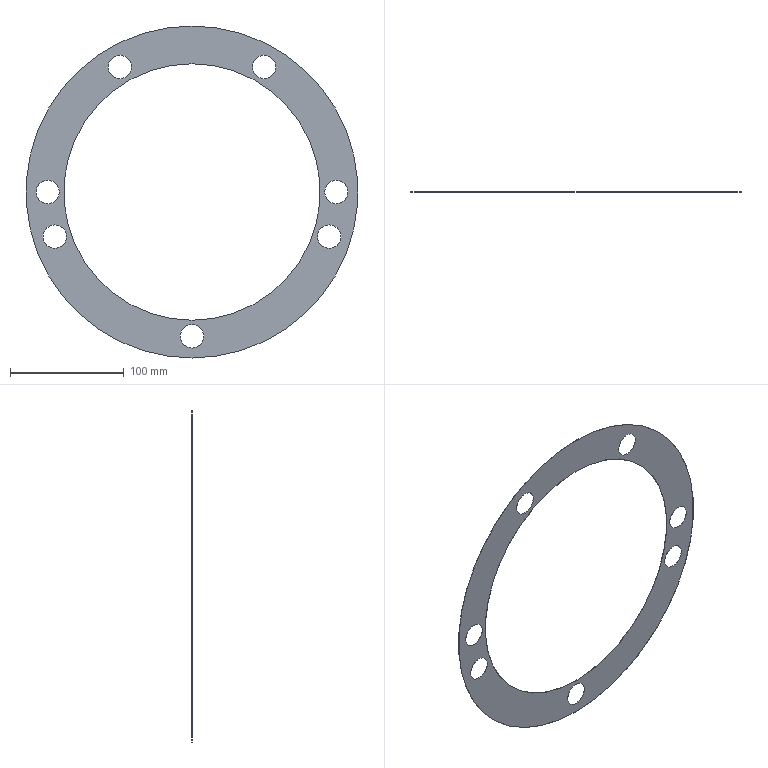Part | SolidWorks | features HoleWzd 2, Extrusion 1, MirrorPattern 1 | 1 solid | 20 faces | box 292.1 x 0.254 x 292.1 mm | volume 6277 mm3 | cylinder 18 | plane 2 | commonest cylinder face diameters 20.637 x14 225.552 x2 292.1 x2
STEP:
#1=CARTESIAN_POINT('',(-63.5,0.254,120.301));
#2=VERTEX_POINT('',#1);
#3=CARTESIAN_POINT('',(-63.5,0.254,99.663));
#4=VERTEX_POINT('',#3);
#5=CARTESIAN_POINT('',(-63.5,0.254,109.982));
#6=DIRECTION('',(0.,-1.,0.));
#7=DIRECTION('',(0.,0.,-1.));
#8=AXIS2_PLACEMENT_3D('',#5,#6,#7);
#9=CIRCLE('',#8,10.319);
#10=EDGE_CURVE('',#2,#4,#9,.T.);
#11=ORIENTED_EDGE('',*,*,#10,.F.);
#12=CARTESIAN_POINT('',(-63.5,0.,120.301));
#13=VERTEX_POINT('',#12);
#14=CARTESIAN_POINT('',(-63.5,0.,120.301));
#15=DIRECTION('',(0.,-1.,0.));
#16=VECTOR('',#15,1000.);
#17=LINE('',#14,#16);
#18=EDGE_CURVE('',#2,#13,#17,.T.);
#19=ORIENTED_EDGE('',*,*,#18,.T.);
#20=CARTESIAN_POINT('',(-63.5,0.,99.663));
#21=VERTEX_POINT('',#20);
#22=CARTESIAN_POINT('',(-63.5,0.,109.982));
#23=DIRECTION('',(0.,-1.,0.));
#24=DIRECTION('',(0.,0.,-1.));
#25=AXIS2_PLACEMENT_3D('',#22,#23,#24);
#26=CIRCLE('',#25,10.319);
#27=EDGE_CURVE('',#13,#21,#26,.T.);
#28=ORIENTED_EDGE('',*,*,#27,.T.);
#29=CARTESIAN_POINT('',(-63.5,0.,99.663));
#30=DIRECTION('',(0.,-1.,0.));
#31=VECTOR('',#30,1000.);
#32=LINE('',#29,#31);
#33=EDGE_CURVE('',#4,#21,#32,.T.);
#34=ORIENTED_EDGE('',*,*,#33,.F.);
#35=EDGE_LOOP('',(#11,#19,#28,#34));
#36=FACE_OUTER_BOUND('',#35,.T.);
#37=CARTESIAN_POINT('',(-63.5,0.,109.982));
#38=DIRECTION('',(0.,-1.,0.));
#39=DIRECTION('',(0.,0.,-1.));
#40=AXIS2_PLACEMENT_3D('',#37,#38,#39);
#41=CYLINDRICAL_SURFACE('',#40,10.319);
#42=ADVANCED_FACE('',(#36),#41,.F.);
#43=CARTESIAN_POINT('',(-120.77,0.254,-28.924));
#44=VERTEX_POINT('',#43);
#45=CARTESIAN_POINT('',(-120.77,0.254,-49.562));
#46=VERTEX_POINT('',#45);
#47=CARTESIAN_POINT('',(-120.77,0.254,-39.243));
#48=DIRECTION('',(0.,-1.,0.));
#49=DIRECTION('',(0.,0.,-1.));
#50=AXIS2_PLACEMENT_3D('',#47,#48,#49);
#51=CIRCLE('',#50,10.319);
#52=EDGE_CURVE('',#44,#46,#51,.T.);
#53=ORIENTED_EDGE('',*,*,#52,.F.);
#54=CARTESIAN_POINT('',(-120.77,0.,-28.924));
#55=VERTEX_POINT('',#54);
#56=CARTESIAN_POINT('',(-120.77,0.,-28.924));
#57=DIRECTION('',(0.,-1.,0.));
#58=VECTOR('',#57,1000.);
#59=LINE('',#56,#58);
#60=EDGE_CURVE('',#44,#55,#59,.T.);
#61=ORIENTED_EDGE('',*,*,#60,.T.);
#62=CARTESIAN_POINT('',(-120.77,0.,-49.562));
#63=VERTEX_POINT('',#62);
#64=CARTESIAN_POINT('',(-120.77,0.,-39.243));
#65=DIRECTION('',(0.,-1.,0.));
#66=DIRECTION('',(0.,0.,-1.));
#67=AXIS2_PLACEMENT_3D('',#64,#65,#66);
#68=CIRCLE('',#67,10.319);
#69=EDGE_CURVE('',#55,#63,#68,.T.);
#70=ORIENTED_EDGE('',*,*,#69,.T.);
#71=CARTESIAN_POINT('',(-120.77,0.,-49.562));
#72=DIRECTION('',(0.,-1.,0.));
#73=VECTOR('',#72,1000.);
#74=LINE('',#71,#73);
#75=EDGE_CURVE('',#46,#63,#74,.T.);
#76=ORIENTED_EDGE('',*,*,#75,.F.);
#77=EDGE_LOOP('',(#53,#61,#70,#76));
#78=FACE_OUTER_BOUND('',#77,.T.);
#79=CARTESIAN_POINT('',(-120.77,0.,-39.243));
#80=DIRECTION('',(0.,-1.,0.));
#81=DIRECTION('',(0.,0.,-1.));
#82=AXIS2_PLACEMENT_3D('',#79,#80,#81);
#83=CYLINDRICAL_SURFACE('',#82,10.319);
#84=ADVANCED_FACE('',(#78),#83,.F.);
#85=CARTESIAN_POINT('',(-127.,0.254,10.319));
#86=VERTEX_POINT('',#85);
#87=CARTESIAN_POINT('',(-127.,0.254,-10.319));
#88=VERTEX_POINT('',#87);
#89=CARTESIAN_POINT('',(-127.,0.254,0.));
#90=DIRECTION('',(0.,-1.,0.));
#91=DIRECTION('',(0.,0.,-1.));
#92=AXIS2_PLACEMENT_3D('',#89,#90,#91);
#93=CIRCLE('',#92,10.319);
#94=EDGE_CURVE('',#86,#88,#93,.T.);
#95=ORIENTED_EDGE('',*,*,#94,.F.);
#96=CARTESIAN_POINT('',(-127.,0.,10.319));
#97=VERTEX_POINT('',#96);
#98=CARTESIAN_POINT('',(-127.,0.,10.319));
#99=DIRECTION('',(0.,-1.,0.));
#100=VECTOR('',#99,1000.);
#101=LINE('',#98,#100);
#102=EDGE_CURVE('',#86,#97,#101,.T.);
#103=ORIENTED_EDGE('',*,*,#102,.T.);
#104=CARTESIAN_POINT('',(-127.,0.,-10.319));
#105=VERTEX_POINT('',#104);
#106=CARTESIAN_POINT('',(-127.,0.,0.));
#107=DIRECTION('',(0.,-1.,0.));
#108=DIRECTION('',(0.,0.,-1.));
#109=AXIS2_PLACEMENT_3D('',#106,#107,#108);
#110=CIRCLE('',#109,10.319);
#111=EDGE_CURVE('',#97,#105,#110,.T.);
#112=ORIENTED_EDGE('',*,*,#111,.T.);
#113=CARTESIAN_POINT('',(-127.,0.,-10.319));
#114=DIRECTION('',(0.,-1.,0.));
#115=VECTOR('',#114,1000.);
#116=LINE('',#113,#115);
#117=EDGE_CURVE('',#88,#105,#116,.T.);
#118=ORIENTED_EDGE('',*,*,#117,.F.);
#119=EDGE_LOOP('',(#95,#103,#112,#118));
#120=FACE_OUTER_BOUND('',#119,.T.);
#121=CARTESIAN_POINT('',(-127.,0.,0.));
#122=DIRECTION('',(0.,-1.,0.));
#123=DIRECTION('',(0.,0.,-1.));
#124=AXIS2_PLACEMENT_3D('',#121,#122,#123);
#125=CYLINDRICAL_SURFACE('',#124,10.319);
#126=ADVANCED_FACE('',(#120),#125,.F.);
#127=CARTESIAN_POINT('',(63.5,0.254,120.301));
#128=VERTEX_POINT('',#127);
#129=CARTESIAN_POINT('',(63.5,0.254,99.663));
#130=VERTEX_POINT('',#129);
#131=CARTESIAN_POINT('',(63.5,0.254,109.982));
#132=DIRECTION('',(0.,-1.,0.));
#133=DIRECTION('',(0.,0.,-1.));
#134=AXIS2_PLACEMENT_3D('',#131,#132,#133);
#135=CIRCLE('',#134,10.319);
#136=EDGE_CURVE('',#128,#130,#135,.T.);
#137=ORIENTED_EDGE('',*,*,#136,.F.);
#138=CARTESIAN_POINT('',(63.5,0.,120.301));
#139=VERTEX_POINT('',#138);
#140=CARTESIAN_POINT('',(63.5,0.,120.301));
#141=DIRECTION('',(0.,-1.,0.));
#142=VECTOR('',#141,1000.);
#143=LINE('',#140,#142);
#144=EDGE_CURVE('',#128,#139,#143,.T.);
#145=ORIENTED_EDGE('',*,*,#144,.T.);
#146=CARTESIAN_POINT('',(63.5,0.,99.663));
#147=VERTEX_POINT('',#146);
#148=CARTESIAN_POINT('',(63.5,0.,109.982));
#149=DIRECTION('',(0.,-1.,0.));
#150=DIRECTION('',(0.,0.,-1.));
#151=AXIS2_PLACEMENT_3D('',#148,#149,#150);
#152=CIRCLE('',#151,10.319);
#153=EDGE_CURVE('',#139,#147,#152,.T.);
#154=ORIENTED_EDGE('',*,*,#153,.T.);
#155=CARTESIAN_POINT('',(63.5,0.,99.663));
#156=DIRECTION('',(0.,-1.,0.));
#157=VECTOR('',#156,1000.);
#158=LINE('',#155,#157);
#159=EDGE_CURVE('',#130,#147,#158,.T.);
#160=ORIENTED_EDGE('',*,*,#159,.F.);
#161=EDGE_LOOP('',(#137,#145,#154,#160));
#162=FACE_OUTER_BOUND('',#161,.T.);
#163=CARTESIAN_POINT('',(63.5,0.,109.982));
#164=DIRECTION('',(0.,-1.,0.));
#165=DIRECTION('',(0.,0.,-1.));
#166=AXIS2_PLACEMENT_3D('',#163,#164,#165);
#167=CYLINDRICAL_SURFACE('',#166,10.319);
#168=ADVANCED_FACE('',(#162),#167,.F.);
#169=CARTESIAN_POINT('',(120.77,0.254,-28.924));
#170=VERTEX_POINT('',#169);
#171=CARTESIAN_POINT('',(120.77,0.254,-49.562));
#172=VERTEX_POINT('',#171);
#173=CARTESIAN_POINT('',(120.77,0.254,-39.243));
#174=DIRECTION('',(0.,-1.,0.));
#175=DIRECTION('',(0.,0.,-1.));
#176=AXIS2_PLACEMENT_3D('',#173,#174,#175);
#177=CIRCLE('',#176,10.319);
#178=EDGE_CURVE('',#170,#172,#177,.T.);
#179=ORIENTED_EDGE('',*,*,#178,.F.);
#180=CARTESIAN_POINT('',(120.77,0.,-28.924));
#181=VERTEX_POINT('',#180);
#182=CARTESIAN_POINT('',(120.77,0.,-28.924));
#183=DIRECTION('',(0.,-1.,0.));
#184=VECTOR('',#183,1000.);
#185=LINE('',#182,#184);
#186=EDGE_CURVE('',#170,#181,#185,.T.);
#187=ORIENTED_EDGE('',*,*,#186,.T.);
#188=CARTESIAN_POINT('',(120.77,0.,-49.562));
#189=VERTEX_POINT('',#188);
#190=CARTESIAN_POINT('',(120.77,0.,-39.243));
#191=DIRECTION('',(0.,-1.,0.));
#192=DIRECTION('',(0.,0.,-1.));
#193=AXIS2_PLACEMENT_3D('',#190,#191,#192);
#194=CIRCLE('',#193,10.319);
#195=EDGE_CURVE('',#181,#189,#194,.T.);
#196=ORIENTED_EDGE('',*,*,#195,.T.);
#197=CARTESIAN_POINT('',(120.77,0.,-49.562));
#198=DIRECTION('',(0.,-1.,0.));
#199=VECTOR('',#198,1000.);
#200=LINE('',#197,#199);
#201=EDGE_CURVE('',#172,#189,#200,.T.);
#202=ORIENTED_EDGE('',*,*,#201,.F.);
#203=EDGE_LOOP('',(#179,#187,#196,#202));
#204=FACE_OUTER_BOUND('',#203,.T.);
#205=CARTESIAN_POINT('',(120.77,0.,-39.243));
#206=DIRECTION('',(0.,-1.,0.));
#207=DIRECTION('',(0.,0.,-1.));
#208=AXIS2_PLACEMENT_3D('',#205,#206,#207);
#209=CYLINDRICAL_SURFACE('',#208,10.319);
#210=ADVANCED_FACE('',(#204),#209,.F.);
#211=CARTESIAN_POINT('',(127.,0.254,10.319));
#212=VERTEX_POINT('',#211);
#213=CARTESIAN_POINT('',(127.,0.254,-10.319));
#214=VERTEX_POINT('',#213);
#215=CARTESIAN_POINT('',(127.,0.254,0.));
#216=DIRECTION('',(0.,-1.,0.));
#217=DIRECTION('',(0.,0.,-1.));
#218=AXIS2_PLACEMENT_3D('',#215,#216,#217);
#219=CIRCLE('',#218,10.319);
#220=EDGE_CURVE('',#212,#214,#219,.T.);
#221=ORIENTED_EDGE('',*,*,#220,.F.);
#222=CARTESIAN_POINT('',(127.,0.,10.319));
#223=VERTEX_POINT('',#222);
#224=CARTESIAN_POINT('',(127.,0.,10.319));
#225=DIRECTION('',(0.,-1.,0.));
#226=VECTOR('',#225,1000.);
#227=LINE('',#224,#226);
#228=EDGE_CURVE('',#212,#223,#227,.T.);
#229=ORIENTED_EDGE('',*,*,#228,.T.);
#230=CARTESIAN_POINT('',(127.,0.,-10.319));
#231=VERTEX_POINT('',#230);
#232=CARTESIAN_POINT('',(127.,0.,0.));
#233=DIRECTION('',(0.,-1.,0.));
#234=DIRECTION('',(0.,0.,-1.));
#235=AXIS2_PLACEMENT_3D('',#232,#233,#234);
#236=CIRCLE('',#235,10.319);
#237=EDGE_CURVE('',#223,#231,#236,.T.);
#238=ORIENTED_EDGE('',*,*,#237,.T.);
#239=CARTESIAN_POINT('',(127.,0.,-10.319));
#240=DIRECTION('',(0.,-1.,0.));
#241=VECTOR('',#240,1000.);
#242=LINE('',#239,#241);
#243=EDGE_CURVE('',#214,#231,#242,.T.);
#244=ORIENTED_EDGE('',*,*,#243,.F.);
#245=EDGE_LOOP('',(#221,#229,#238,#244));
#246=FACE_OUTER_BOUND('',#245,.T.);
#247=CARTESIAN_POINT('',(127.,0.,0.));
#248=DIRECTION('',(0.,-1.,0.));
#249=DIRECTION('',(0.,0.,-1.));
#250=AXIS2_PLACEMENT_3D('',#247,#248,#249);
#251=CYLINDRICAL_SURFACE('',#250,10.319);
#252=ADVANCED_FACE('',(#246),#251,.F.);
#253=CARTESIAN_POINT('',(0.,0.,-137.319));
#254=VERTEX_POINT('',#253);
#255=CARTESIAN_POINT('',(0.,0.,-116.681));
#256=VERTEX_POINT('',#255);
#257=CARTESIAN_POINT('',(0.,0.,-127.));
#258=DIRECTION('',(0.,1.,0.));
#259=DIRECTION('',(0.,0.,1.));
#260=AXIS2_PLACEMENT_3D('',#257,#258,#259);
#261=CIRCLE('',#260,10.319);
#262=EDGE_CURVE('',#254,#256,#261,.T.);
#263=ORIENTED_EDGE('',*,*,#262,.F.);
#264=CARTESIAN_POINT('',(0.,0.254,-137.319));
#265=VERTEX_POINT('',#264);
#266=CARTESIAN_POINT('',(0.,0.254,-137.319));
#267=DIRECTION('',(0.,1.,0.));
#268=VECTOR('',#267,1000.);
#269=LINE('',#266,#268);
#270=EDGE_CURVE('',#254,#265,#269,.T.);
#271=ORIENTED_EDGE('',*,*,#270,.T.);
#272=CARTESIAN_POINT('',(0.,0.254,-116.681));
#273=VERTEX_POINT('',#272);
#274=CARTESIAN_POINT('',(0.,0.254,-127.));
#275=DIRECTION('',(0.,1.,0.));
#276=DIRECTION('',(0.,0.,1.));
#277=AXIS2_PLACEMENT_3D('',#274,#275,#276);
#278=CIRCLE('',#277,10.319);
#279=EDGE_CURVE('',#265,#273,#278,.T.);
#280=ORIENTED_EDGE('',*,*,#279,.T.);
#281=CARTESIAN_POINT('',(0.,0.254,-116.681));
#282=DIRECTION('',(0.,1.,0.));
#283=VECTOR('',#282,1000.);
#284=LINE('',#281,#283);
#285=EDGE_CURVE('',#256,#273,#284,.T.);
#286=ORIENTED_EDGE('',*,*,#285,.F.);
#287=EDGE_LOOP('',(#263,#271,#280,#286));
#288=FACE_OUTER_BOUND('',#287,.T.);
#289=CARTESIAN_POINT('',(0.,0.254,-127.));
#290=DIRECTION('',(0.,1.,0.));
#291=DIRECTION('',(0.,0.,1.));
#292=AXIS2_PLACEMENT_3D('',#289,#290,#291);
#293=CYLINDRICAL_SURFACE('',#292,10.319);
#294=ADVANCED_FACE('',(#288),#293,.F.);
#295=CARTESIAN_POINT('',(0.,0.254,-112.776));
#296=VERTEX_POINT('',#295);
#297=CARTESIAN_POINT('',(0.,0.254,112.776));
#298=VERTEX_POINT('',#297);
#299=CARTESIAN_POINT('',(0.,0.254,0.));
#300=DIRECTION('',(0.,1.,0.));
#301=DIRECTION('',(0.,0.,1.));
#302=AXIS2_PLACEMENT_3D('',#299,#300,#301);
#303=CIRCLE('',#302,112.776);
#304=EDGE_CURVE('',#296,#298,#303,.T.);
#305=ORIENTED_EDGE('',*,*,#304,.T.);
#306=CARTESIAN_POINT('',(0.,0.,112.776));
#307=VERTEX_POINT('',#306);
#308=CARTESIAN_POINT('',(0.,0.254,112.776));
#309=DIRECTION('',(0.,-1.,0.));
#310=VECTOR('',#309,1000.);
#311=LINE('',#308,#310);
#312=EDGE_CURVE('',#298,#307,#311,.T.);
#313=ORIENTED_EDGE('',*,*,#312,.T.);
#314=CARTESIAN_POINT('',(0.,0.,-112.776));
#315=VERTEX_POINT('',#314);
#316=CARTESIAN_POINT('',(0.,0.,0.));
#317=DIRECTION('',(0.,1.,0.));
#318=DIRECTION('',(0.,0.,1.));
#319=AXIS2_PLACEMENT_3D('',#316,#317,#318);
#320=CIRCLE('',#319,112.776);
#321=EDGE_CURVE('',#315,#307,#320,.T.);
#322=ORIENTED_EDGE('',*,*,#321,.F.);
#323=CARTESIAN_POINT('',(0.,0.254,-112.776));
#324=DIRECTION('',(0.,-1.,0.));
#325=VECTOR('',#324,1000.);
#326=LINE('',#323,#325);
#327=EDGE_CURVE('',#296,#315,#326,.T.);
#328=ORIENTED_EDGE('',*,*,#327,.F.);
#329=EDGE_LOOP('',(#305,#313,#322,#328));
#330=FACE_OUTER_BOUND('',#329,.T.);
#331=CARTESIAN_POINT('',(0.,0.254,0.));
#332=DIRECTION('',(0.,-1.,0.));
#333=DIRECTION('',(0.,0.,-1.));
#334=AXIS2_PLACEMENT_3D('',#331,#332,#333);
#335=CYLINDRICAL_SURFACE('',#334,112.776);
#336=ADVANCED_FACE('',(#330),#335,.F.);
#337=CARTESIAN_POINT('',(0.,0.254,146.05));
#338=VERTEX_POINT('',#337);
#339=CARTESIAN_POINT('',(0.,0.254,-146.05));
#340=VERTEX_POINT('',#339);
#341=CARTESIAN_POINT('',(0.,0.254,0.));
#342=DIRECTION('',(0.,1.,0.));
#343=DIRECTION('',(0.,0.,1.));
#344=AXIS2_PLACEMENT_3D('',#341,#342,#343);
#345=CIRCLE('',#344,146.05);
#346=EDGE_CURVE('',#338,#340,#345,.T.);
#347=ORIENTED_EDGE('',*,*,#346,.F.);
#348=CARTESIAN_POINT('',(0.,0.,146.05));
#349=VERTEX_POINT('',#348);
#350=CARTESIAN_POINT('',(0.,0.254,146.05));
#351=DIRECTION('',(0.,-1.,0.));
#352=VECTOR('',#351,1000.);
#353=LINE('',#350,#352);
#354=EDGE_CURVE('',#338,#349,#353,.T.);
#355=ORIENTED_EDGE('',*,*,#354,.T.);
#356=CARTESIAN_POINT('',(0.,0.,-146.05));
#357=VERTEX_POINT('',#356);
#358=CARTESIAN_POINT('',(0.,0.,0.));
#359=DIRECTION('',(0.,1.,0.));
#360=DIRECTION('',(0.,0.,1.));
#361=AXIS2_PLACEMENT_3D('',#358,#359,#360);
#362=CIRCLE('',#361,146.05);
#363=EDGE_CURVE('',#349,#357,#362,.T.);
#364=ORIENTED_EDGE('',*,*,#363,.T.);
#365=CARTESIAN_POINT('',(0.,0.254,-146.05));
#366=DIRECTION('',(0.,-1.,0.));
#367=VECTOR('',#366,1000.);
#368=LINE('',#365,#367);
#369=EDGE_CURVE('',#340,#357,#368,.T.);
#370=ORIENTED_EDGE('',*,*,#369,.F.);
#371=EDGE_LOOP('',(#347,#355,#364,#370));
#372=FACE_OUTER_BOUND('',#371,.T.);
#373=CARTESIAN_POINT('',(0.,0.254,0.));
#374=DIRECTION('',(0.,-1.,0.));
#375=DIRECTION('',(0.,0.,-1.));
#376=AXIS2_PLACEMENT_3D('',#373,#374,#375);
#377=CYLINDRICAL_SURFACE('',#376,146.05);
#378=ADVANCED_FACE('',(#372),#377,.T.);
#379=CARTESIAN_POINT('',(-120.77,0.,-39.243));
#380=DIRECTION('',(0.,-1.,0.));
#381=DIRECTION('',(0.,0.,-1.));
#382=AXIS2_PLACEMENT_3D('',#379,#380,#381);
#383=CIRCLE('',#382,10.319);
#384=EDGE_CURVE('',#63,#55,#383,.T.);
#385=ORIENTED_EDGE('',*,*,#384,.F.);
#386=ORIENTED_EDGE('',*,*,#69,.F.);
#387=EDGE_LOOP('',(#385,#386));
#388=FACE_BOUND('',#387,.T.);
#389=ORIENTED_EDGE('',*,*,#321,.T.);
#390=CARTESIAN_POINT('',(0.,0.,0.));
#391=DIRECTION('',(0.,1.,0.));
#392=DIRECTION('',(0.,0.,1.));
#393=AXIS2_PLACEMENT_3D('',#390,#391,#392);
#394=CIRCLE('',#393,112.776);
#395=EDGE_CURVE('',#307,#315,#394,.T.);
#396=ORIENTED_EDGE('',*,*,#395,.T.);
#397=EDGE_LOOP('',(#389,#396));
#398=FACE_BOUND('',#397,.T.);
#399=CARTESIAN_POINT('',(0.,0.,0.));
#400=DIRECTION('',(0.,1.,0.));
#401=DIRECTION('',(0.,0.,1.));
#402=AXIS2_PLACEMENT_3D('',#399,#400,#401);
#403=CIRCLE('',#402,146.05);
#404=EDGE_CURVE('',#357,#349,#403,.T.);
#405=ORIENTED_EDGE('',*,*,#404,.F.);
#406=ORIENTED_EDGE('',*,*,#363,.F.);
#407=EDGE_LOOP('',(#405,#406));
#408=FACE_OUTER_BOUND('',#407,.T.);
#409=CARTESIAN_POINT('',(0.,0.,-127.));
#410=DIRECTION('',(0.,1.,0.));
#411=DIRECTION('',(0.,0.,1.));
#412=AXIS2_PLACEMENT_3D('',#409,#410,#411);
#413=CIRCLE('',#412,10.319);
#414=EDGE_CURVE('',#256,#254,#413,.T.);
#415=ORIENTED_EDGE('',*,*,#414,.T.);
#416=ORIENTED_EDGE('',*,*,#262,.T.);
#417=EDGE_LOOP('',(#415,#416));
#418=FACE_BOUND('',#417,.T.);
#419=CARTESIAN_POINT('',(127.,0.,0.));
#420=DIRECTION('',(0.,-1.,0.));
#421=DIRECTION('',(0.,0.,-1.));
#422=AXIS2_PLACEMENT_3D('',#419,#420,#421);
#423=CIRCLE('',#422,10.319);
#424=EDGE_CURVE('',#231,#223,#423,.T.);
#425=ORIENTED_EDGE('',*,*,#424,.F.);
#426=ORIENTED_EDGE('',*,*,#237,.F.);
#427=EDGE_LOOP('',(#425,#426));
#428=FACE_BOUND('',#427,.T.);
#429=CARTESIAN_POINT('',(120.77,0.,-39.243));
#430=DIRECTION('',(0.,-1.,0.));
#431=DIRECTION('',(0.,0.,-1.));
#432=AXIS2_PLACEMENT_3D('',#429,#430,#431);
#433=CIRCLE('',#432,10.319);
#434=EDGE_CURVE('',#189,#181,#433,.T.);
#435=ORIENTED_EDGE('',*,*,#434,.F.);
#436=ORIENTED_EDGE('',*,*,#195,.F.);
#437=EDGE_LOOP('',(#435,#436));
#438=FACE_BOUND('',#437,.T.);
#439=CARTESIAN_POINT('',(63.5,0.,109.982));
#440=DIRECTION('',(0.,-1.,0.));
#441=DIRECTION('',(0.,0.,-1.));
#442=AXIS2_PLACEMENT_3D('',#439,#440,#441);
#443=CIRCLE('',#442,10.319);
#444=EDGE_CURVE('',#147,#139,#443,.T.);
#445=ORIENTED_EDGE('',*,*,#444,.F.);
#446=ORIENTED_EDGE('',*,*,#153,.F.);
#447=EDGE_LOOP('',(#445,#446));
#448=FACE_BOUND('',#447,.T.);
#449=CARTESIAN_POINT('',(-127.,0.,0.));
#450=DIRECTION('',(0.,-1.,0.));
#451=DIRECTION('',(0.,0.,-1.));
#452=AXIS2_PLACEMENT_3D('',#449,#450,#451);
#453=CIRCLE('',#452,10.319);
#454=EDGE_CURVE('',#105,#97,#453,.T.);
#455=ORIENTED_EDGE('',*,*,#454,.F.);
#456=ORIENTED_EDGE('',*,*,#111,.F.);
#457=EDGE_LOOP('',(#455,#456));
#458=FACE_BOUND('',#457,.T.);
#459=CARTESIAN_POINT('',(-63.5,0.,109.982));
#460=DIRECTION('',(0.,-1.,0.));
#461=DIRECTION('',(0.,0.,-1.));
#462=AXIS2_PLACEMENT_3D('',#459,#460,#461);
#463=CIRCLE('',#462,10.319);
#464=EDGE_CURVE('',#21,#13,#463,.T.);
#465=ORIENTED_EDGE('',*,*,#464,.F.);
#466=ORIENTED_EDGE('',*,*,#27,.F.);
#467=EDGE_LOOP('',(#465,#466));
#468=FACE_BOUND('',#467,.T.);
#469=CARTESIAN_POINT('',(0.,0.,0.));
#470=DIRECTION('',(0.,1.,0.));
#471=DIRECTION('',(0.,0.,1.));
#472=AXIS2_PLACEMENT_3D('',#469,#470,#471);
#473=PLANE('',#472);
#474=ADVANCED_FACE('',(#388,#398,#408,#418,#428,#438,#448,#458,#468),#473,.F.);
#475=CARTESIAN_POINT('',(-120.77,0.254,-39.243));
#476=DIRECTION('',(0.,-1.,0.));
#477=DIRECTION('',(0.,0.,-1.));
#478=AXIS2_PLACEMENT_3D('',#475,#476,#477);
#479=CIRCLE('',#478,10.319);
#480=EDGE_CURVE('',#46,#44,#479,.T.);
#481=ORIENTED_EDGE('',*,*,#480,.T.);
#482=ORIENTED_EDGE('',*,*,#52,.T.);
#483=EDGE_LOOP('',(#481,#482));
#484=FACE_BOUND('',#483,.T.);
#485=CARTESIAN_POINT('',(-127.,0.254,0.));
#486=DIRECTION('',(0.,-1.,0.));
#487=DIRECTION('',(0.,0.,-1.));
#488=AXIS2_PLACEMENT_3D('',#485,#486,#487);
#489=CIRCLE('',#488,10.319);
#490=EDGE_CURVE('',#88,#86,#489,.T.);
#491=ORIENTED_EDGE('',*,*,#490,.T.);
#492=ORIENTED_EDGE('',*,*,#94,.T.);
#493=EDGE_LOOP('',(#491,#492));
#494=FACE_BOUND('',#493,.T.);
#495=CARTESIAN_POINT('',(63.5,0.254,109.982));
#496=DIRECTION('',(0.,-1.,0.));
#497=DIRECTION('',(0.,0.,-1.));
#498=AXIS2_PLACEMENT_3D('',#495,#496,#497);
#499=CIRCLE('',#498,10.319);
#500=EDGE_CURVE('',#130,#128,#499,.T.);
#501=ORIENTED_EDGE('',*,*,#500,.T.);
#502=ORIENTED_EDGE('',*,*,#136,.T.);
#503=EDGE_LOOP('',(#501,#502));
#504=FACE_BOUND('',#503,.T.);
#505=CARTESIAN_POINT('',(120.77,0.254,-39.243));
#506=DIRECTION('',(0.,-1.,0.));
#507=DIRECTION('',(0.,0.,-1.));
#508=AXIS2_PLACEMENT_3D('',#505,#506,#507);
#509=CIRCLE('',#508,10.319);
#510=EDGE_CURVE('',#172,#170,#509,.T.);
#511=ORIENTED_EDGE('',*,*,#510,.T.);
#512=ORIENTED_EDGE('',*,*,#178,.T.);
#513=EDGE_LOOP('',(#511,#512));
#514=FACE_BOUND('',#513,.T.);
#515=CARTESIAN_POINT('',(127.,0.254,0.));
#516=DIRECTION('',(0.,-1.,0.));
#517=DIRECTION('',(0.,0.,-1.));
#518=AXIS2_PLACEMENT_3D('',#515,#516,#517);
#519=CIRCLE('',#518,10.319);
#520=EDGE_CURVE('',#214,#212,#519,.T.);
#521=ORIENTED_EDGE('',*,*,#520,.T.);
#522=ORIENTED_EDGE('',*,*,#220,.T.);
#523=EDGE_LOOP('',(#521,#522));
#524=FACE_BOUND('',#523,.T.);
#525=CARTESIAN_POINT('',(0.,0.254,-127.));
#526=DIRECTION('',(0.,1.,0.));
#527=DIRECTION('',(0.,0.,1.));
#528=AXIS2_PLACEMENT_3D('',#525,#526,#527);
#529=CIRCLE('',#528,10.319);
#530=EDGE_CURVE('',#273,#265,#529,.T.);
#531=ORIENTED_EDGE('',*,*,#530,.F.);
#532=ORIENTED_EDGE('',*,*,#279,.F.);
#533=EDGE_LOOP('',(#531,#532));
#534=FACE_BOUND('',#533,.T.);
#535=CARTESIAN_POINT('',(0.,0.254,0.));
#536=DIRECTION('',(0.,1.,0.));
#537=DIRECTION('',(0.,0.,1.));
#538=AXIS2_PLACEMENT_3D('',#535,#536,#537);
#539=CIRCLE('',#538,146.05);
#540=EDGE_CURVE('',#340,#338,#539,.T.);
#541=ORIENTED_EDGE('',*,*,#540,.T.);
#542=ORIENTED_EDGE('',*,*,#346,.T.);
#543=EDGE_LOOP('',(#541,#542));
#544=FACE_OUTER_BOUND('',#543,.T.);
#545=ORIENTED_EDGE('',*,*,#304,.F.);
#546=CARTESIAN_POINT('',(0.,0.254,0.));
#547=DIRECTION('',(0.,1.,0.));
#548=DIRECTION('',(0.,0.,1.));
#549=AXIS2_PLACEMENT_3D('',#546,#547,#548);
#550=CIRCLE('',#549,112.776);
#551=EDGE_CURVE('',#298,#296,#550,.T.);
#552=ORIENTED_EDGE('',*,*,#551,.F.);
#553=EDGE_LOOP('',(#545,#552));
#554=FACE_BOUND('',#553,.T.);
#555=CARTESIAN_POINT('',(-63.5,0.254,109.982));
#556=DIRECTION('',(0.,-1.,0.));
#557=DIRECTION('',(0.,0.,-1.));
#558=AXIS2_PLACEMENT_3D('',#555,#556,#557);
#559=CIRCLE('',#558,10.319);
#560=EDGE_CURVE('',#4,#2,#559,.T.);
#561=ORIENTED_EDGE('',*,*,#560,.T.);
#562=ORIENTED_EDGE('',*,*,#10,.T.);
#563=EDGE_LOOP('',(#561,#562));
#564=FACE_BOUND('',#563,.T.);
#565=CARTESIAN_POINT('',(0.,0.254,0.));
#566=DIRECTION('',(0.,1.,0.));
#567=DIRECTION('',(0.,0.,1.));
#568=AXIS2_PLACEMENT_3D('',#565,#566,#567);
#569=PLANE('',#568);
#570=ADVANCED_FACE('',(#484,#494,#504,#514,#524,#534,#544,#554,#564),#569,.T.);
#571=ORIENTED_EDGE('',*,*,#354,.F.);
#572=ORIENTED_EDGE('',*,*,#540,.F.);
#573=ORIENTED_EDGE('',*,*,#369,.T.);
#574=ORIENTED_EDGE('',*,*,#404,.T.);
#575=EDGE_LOOP('',(#571,#572,#573,#574));
#576=FACE_OUTER_BOUND('',#575,.T.);
#577=CARTESIAN_POINT('',(0.,0.254,0.));
#578=DIRECTION('',(0.,-1.,0.));
#579=DIRECTION('',(0.,0.,-1.));
#580=AXIS2_PLACEMENT_3D('',#577,#578,#579);
#581=CYLINDRICAL_SURFACE('',#580,146.05);
#582=ADVANCED_FACE('',(#576),#581,.T.);
#583=ORIENTED_EDGE('',*,*,#312,.F.);
#584=ORIENTED_EDGE('',*,*,#551,.T.);
#585=ORIENTED_EDGE('',*,*,#327,.T.);
#586=ORIENTED_EDGE('',*,*,#395,.F.);
#587=EDGE_LOOP('',(#583,#584,#585,#586));
#588=FACE_OUTER_BOUND('',#587,.T.);
#589=CARTESIAN_POINT('',(0.,0.254,0.));
#590=DIRECTION('',(0.,-1.,0.));
#591=DIRECTION('',(0.,0.,-1.));
#592=AXIS2_PLACEMENT_3D('',#589,#590,#591);
#593=CYLINDRICAL_SURFACE('',#592,112.776);
#594=ADVANCED_FACE('',(#588),#593,.F.);
#595=ORIENTED_EDGE('',*,*,#270,.F.);
#596=ORIENTED_EDGE('',*,*,#414,.F.);
#597=ORIENTED_EDGE('',*,*,#285,.T.);
#598=ORIENTED_EDGE('',*,*,#530,.T.);
#599=EDGE_LOOP('',(#595,#596,#597,#598));
#600=FACE_OUTER_BOUND('',#599,.T.);
#601=CARTESIAN_POINT('',(0.,0.254,-127.));
#602=DIRECTION('',(0.,1.,0.));
#603=DIRECTION('',(0.,0.,1.));
#604=AXIS2_PLACEMENT_3D('',#601,#602,#603);
#605=CYLINDRICAL_SURFACE('',#604,10.319);
#606=ADVANCED_FACE('',(#600),#605,.F.);
#607=ORIENTED_EDGE('',*,*,#228,.F.);
#608=ORIENTED_EDGE('',*,*,#520,.F.);
#609=ORIENTED_EDGE('',*,*,#243,.T.);
#610=ORIENTED_EDGE('',*,*,#424,.T.);
#611=EDGE_LOOP('',(#607,#608,#609,#610));
#612=FACE_OUTER_BOUND('',#611,.T.);
#613=CARTESIAN_POINT('',(127.,0.,0.));
#614=DIRECTION('',(0.,-1.,0.));
#615=DIRECTION('',(0.,0.,-1.));
#616=AXIS2_PLACEMENT_3D('',#613,#614,#615);
#617=CYLINDRICAL_SURFACE('',#616,10.319);
#618=ADVANCED_FACE('',(#612),#617,.F.);
#619=ORIENTED_EDGE('',*,*,#186,.F.);
#620=ORIENTED_EDGE('',*,*,#510,.F.);
#621=ORIENTED_EDGE('',*,*,#201,.T.);
#622=ORIENTED_EDGE('',*,*,#434,.T.);
#623=EDGE_LOOP('',(#619,#620,#621,#622));
#624=FACE_OUTER_BOUND('',#623,.T.);
#625=CARTESIAN_POINT('',(120.77,0.,-39.243));
#626=DIRECTION('',(0.,-1.,0.));
#627=DIRECTION('',(0.,0.,-1.));
#628=AXIS2_PLACEMENT_3D('',#625,#626,#627);
#629=CYLINDRICAL_SURFACE('',#628,10.319);
#630=ADVANCED_FACE('',(#624),#629,.F.);
#631=ORIENTED_EDGE('',*,*,#144,.F.);
#632=ORIENTED_EDGE('',*,*,#500,.F.);
#633=ORIENTED_EDGE('',*,*,#159,.T.);
#634=ORIENTED_EDGE('',*,*,#444,.T.);
#635=EDGE_LOOP('',(#631,#632,#633,#634));
#636=FACE_OUTER_BOUND('',#635,.T.);
#637=CARTESIAN_POINT('',(63.5,0.,109.982));
#638=DIRECTION('',(0.,-1.,0.));
#639=DIRECTION('',(0.,0.,-1.));
#640=AXIS2_PLACEMENT_3D('',#637,#638,#639);
#641=CYLINDRICAL_SURFACE('',#640,10.319);
#642=ADVANCED_FACE('',(#636),#641,.F.);
#643=ORIENTED_EDGE('',*,*,#102,.F.);
#644=ORIENTED_EDGE('',*,*,#490,.F.);
#645=ORIENTED_EDGE('',*,*,#117,.T.);
#646=ORIENTED_EDGE('',*,*,#454,.T.);
#647=EDGE_LOOP('',(#643,#644,#645,#646));
#648=FACE_OUTER_BOUND('',#647,.T.);
#649=CARTESIAN_POINT('',(-127.,0.,0.));
#650=DIRECTION('',(0.,-1.,0.));
#651=DIRECTION('',(0.,0.,-1.));
#652=AXIS2_PLACEMENT_3D('',#649,#650,#651);
#653=CYLINDRICAL_SURFACE('',#652,10.319);
#654=ADVANCED_FACE('',(#648),#653,.F.);
#655=ORIENTED_EDGE('',*,*,#60,.F.);
#656=ORIENTED_EDGE('',*,*,#480,.F.);
#657=ORIENTED_EDGE('',*,*,#75,.T.);
#658=ORIENTED_EDGE('',*,*,#384,.T.);
#659=EDGE_LOOP('',(#655,#656,#657,#658));
#660=FACE_OUTER_BOUND('',#659,.T.);
#661=CARTESIAN_POINT('',(-120.77,0.,-39.243));
#662=DIRECTION('',(0.,-1.,0.));
#663=DIRECTION('',(0.,0.,-1.));
#664=AXIS2_PLACEMENT_3D('',#661,#662,#663);
#665=CYLINDRICAL_SURFACE('',#664,10.319);
#666=ADVANCED_FACE('',(#660),#665,.F.);
#667=ORIENTED_EDGE('',*,*,#18,.F.);
#668=ORIENTED_EDGE('',*,*,#560,.F.);
#669=ORIENTED_EDGE('',*,*,#33,.T.);
#670=ORIENTED_EDGE('',*,*,#464,.T.);
#671=EDGE_LOOP('',(#667,#668,#669,#670));
#672=FACE_OUTER_BOUND('',#671,.T.);
#673=CARTESIAN_POINT('',(-63.5,0.,109.982));
#674=DIRECTION('',(0.,-1.,0.));
#675=DIRECTION('',(0.,0.,-1.));
#676=AXIS2_PLACEMENT_3D('',#673,#674,#675);
#677=CYLINDRICAL_SURFACE('',#676,10.319);
#678=ADVANCED_FACE('',(#672),#677,.F.);
#679=CLOSED_SHELL('',(#42,#84,#126,#168,#210,#252,#294,#336,#378,#474,#570,#582,#594,#606,#618,#630,#642,#654,#666,#678));
#680=MANIFOLD_SOLID_BREP('',#679);
#681=CARTESIAN_POINT('',(0.,0.,0.));
#682=DIRECTION('',(0.,0.,1.));
#683=DIRECTION('',(1.,0.,0.));
#684=AXIS2_PLACEMENT_3D('',#681,#682,#683);
#685=(LENGTH_UNIT()NAMED_UNIT(*)SI_UNIT(.MILLI.,.METRE.));
#686=UNCERTAINTY_MEASURE_WITH_UNIT(LENGTH_MEASURE(0.00001),#685,'','');
#687=(NAMED_UNIT(*)PLANE_ANGLE_UNIT()SI_UNIT($,.RADIAN.));
#688=(NAMED_UNIT(*)SI_UNIT($,.STERADIAN.)SOLID_ANGLE_UNIT());
#689=(GEOMETRIC_REPRESENTATION_CONTEXT(3)GLOBAL_UNCERTAINTY_ASSIGNED_CONTEXT((#686))GLOBAL_UNIT_ASSIGNED_CONTEXT((#685,#687,#688))REPRESENTATION_CONTEXT('',''));
#690=ADVANCED_BREP_SHAPE_REPRESENTATION('',(#680,#684),#689);